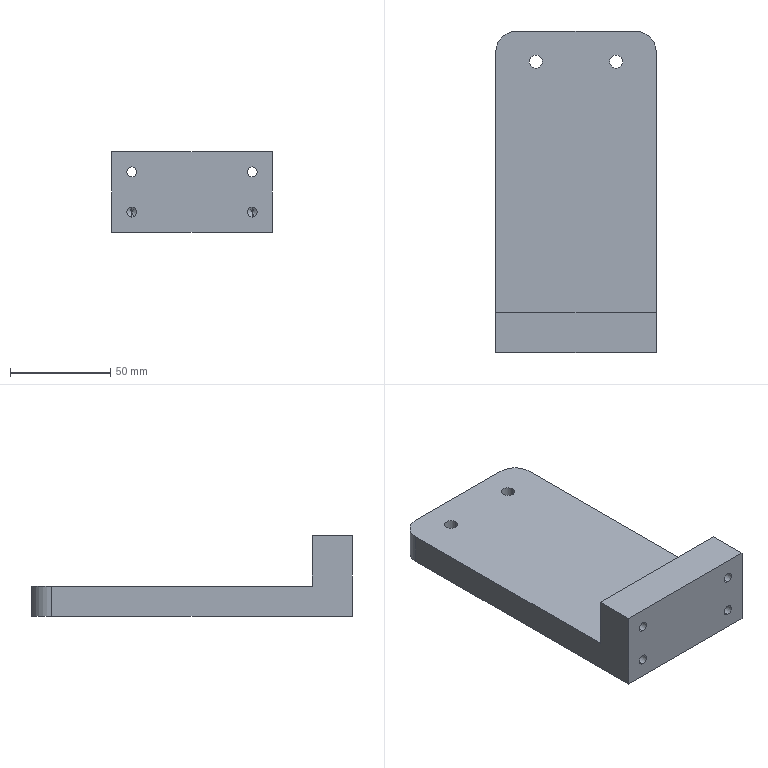Part | SolidWorks | features BaseBody 1 | 1 solid | 32 faces | box 80 x 160 x 40 mm | volume 227794 mm3 | cylinder 18 | plane 10 | cone 4 | commonest cylinder face diameters 5 x8 6.6 x4 11 x4 20 x2
STEP:
#1=CARTESIAN_POINT('',(25.5,65.,6.8));
#2=VERTEX_POINT('',#1);
#3=CARTESIAN_POINT('',(14.5,65.,6.8));
#4=VERTEX_POINT('',#3);
#5=CARTESIAN_POINT('',(20.,65.,6.8));
#6=DIRECTION('',(0.,0.,-1.));
#7=DIRECTION('',(-1.,0.,0.));
#8=AXIS2_PLACEMENT_3D('',#5,#6,#7);
#9=CIRCLE('',#8,5.5);
#10=EDGE_CURVE('',#2,#4,#9,.T.);
#11=ORIENTED_EDGE('',*,*,#10,.F.);
#12=CARTESIAN_POINT('',(25.5,65.,0.));
#13=VERTEX_POINT('',#12);
#14=CARTESIAN_POINT('',(25.5,65.,0.));
#15=DIRECTION('',(0.,0.,-1.));
#16=VECTOR('',#15,1000.);
#17=LINE('',#14,#16);
#18=EDGE_CURVE('',#2,#13,#17,.T.);
#19=ORIENTED_EDGE('',*,*,#18,.T.);
#20=CARTESIAN_POINT('',(14.5,65.,0.));
#21=VERTEX_POINT('',#20);
#22=CARTESIAN_POINT('',(20.,65.,0.));
#23=DIRECTION('',(0.,0.,-1.));
#24=DIRECTION('',(-1.,0.,0.));
#25=AXIS2_PLACEMENT_3D('',#22,#23,#24);
#26=CIRCLE('',#25,5.5);
#27=EDGE_CURVE('',#13,#21,#26,.T.);
#28=ORIENTED_EDGE('',*,*,#27,.T.);
#29=CARTESIAN_POINT('',(14.5,65.,0.));
#30=DIRECTION('',(0.,0.,-1.));
#31=VECTOR('',#30,1000.);
#32=LINE('',#29,#31);
#33=EDGE_CURVE('',#4,#21,#32,.T.);
#34=ORIENTED_EDGE('',*,*,#33,.F.);
#35=EDGE_LOOP('',(#11,#19,#28,#34));
#36=FACE_OUTER_BOUND('',#35,.T.);
#37=CARTESIAN_POINT('',(20.,65.,0.));
#38=DIRECTION('',(0.,0.,-1.));
#39=DIRECTION('',(-1.,0.,0.));
#40=AXIS2_PLACEMENT_3D('',#37,#38,#39);
#41=CYLINDRICAL_SURFACE('',#40,5.5);
#42=ADVANCED_FACE('',(#36),#41,.F.);
#43=CARTESIAN_POINT('',(23.3,65.,15.));
#44=VERTEX_POINT('',#43);
#45=CARTESIAN_POINT('',(16.7,65.,15.));
#46=VERTEX_POINT('',#45);
#47=CARTESIAN_POINT('',(20.,65.,15.));
#48=DIRECTION('',(0.,0.,-1.));
#49=DIRECTION('',(-1.,0.,0.));
#50=AXIS2_PLACEMENT_3D('',#47,#48,#49);
#51=CIRCLE('',#50,3.3);
#52=EDGE_CURVE('',#44,#46,#51,.T.);
#53=ORIENTED_EDGE('',*,*,#52,.F.);
#54=CARTESIAN_POINT('',(23.3,65.,6.8));
#55=VERTEX_POINT('',#54);
#56=CARTESIAN_POINT('',(23.3,65.,0.));
#57=DIRECTION('',(0.,0.,-1.));
#58=VECTOR('',#57,1000.);
#59=LINE('',#56,#58);
#60=EDGE_CURVE('',#44,#55,#59,.T.);
#61=ORIENTED_EDGE('',*,*,#60,.T.);
#62=CARTESIAN_POINT('',(16.7,65.,6.8));
#63=VERTEX_POINT('',#62);
#64=CARTESIAN_POINT('',(20.,65.,6.8));
#65=DIRECTION('',(0.,0.,-1.));
#66=DIRECTION('',(-1.,0.,0.));
#67=AXIS2_PLACEMENT_3D('',#64,#65,#66);
#68=CIRCLE('',#67,3.3);
#69=EDGE_CURVE('',#55,#63,#68,.T.);
#70=ORIENTED_EDGE('',*,*,#69,.T.);
#71=CARTESIAN_POINT('',(16.7,65.,0.));
#72=DIRECTION('',(0.,0.,-1.));
#73=VECTOR('',#72,1000.);
#74=LINE('',#71,#73);
#75=EDGE_CURVE('',#46,#63,#74,.T.);
#76=ORIENTED_EDGE('',*,*,#75,.F.);
#77=EDGE_LOOP('',(#53,#61,#70,#76));
#78=FACE_OUTER_BOUND('',#77,.T.);
#79=CARTESIAN_POINT('',(20.,65.,0.));
#80=DIRECTION('',(0.,0.,-1.));
#81=DIRECTION('',(-1.,0.,0.));
#82=AXIS2_PLACEMENT_3D('',#79,#80,#81);
#83=CYLINDRICAL_SURFACE('',#82,3.3);
#84=ADVANCED_FACE('',(#78),#83,.F.);
#85=CARTESIAN_POINT('',(-14.5,65.,6.8));
#86=VERTEX_POINT('',#85);
#87=CARTESIAN_POINT('',(-25.5,65.,6.8));
#88=VERTEX_POINT('',#87);
#89=CARTESIAN_POINT('',(-20.,65.,6.8));
#90=DIRECTION('',(0.,0.,-1.));
#91=DIRECTION('',(-1.,0.,0.));
#92=AXIS2_PLACEMENT_3D('',#89,#90,#91);
#93=CIRCLE('',#92,5.5);
#94=EDGE_CURVE('',#86,#88,#93,.T.);
#95=ORIENTED_EDGE('',*,*,#94,.F.);
#96=CARTESIAN_POINT('',(-14.5,65.,0.));
#97=VERTEX_POINT('',#96);
#98=CARTESIAN_POINT('',(-14.5,65.,0.));
#99=DIRECTION('',(0.,0.,-1.));
#100=VECTOR('',#99,1000.);
#101=LINE('',#98,#100);
#102=EDGE_CURVE('',#86,#97,#101,.T.);
#103=ORIENTED_EDGE('',*,*,#102,.T.);
#104=CARTESIAN_POINT('',(-25.5,65.,0.));
#105=VERTEX_POINT('',#104);
#106=CARTESIAN_POINT('',(-20.,65.,0.));
#107=DIRECTION('',(0.,0.,-1.));
#108=DIRECTION('',(-1.,0.,0.));
#109=AXIS2_PLACEMENT_3D('',#106,#107,#108);
#110=CIRCLE('',#109,5.5);
#111=EDGE_CURVE('',#97,#105,#110,.T.);
#112=ORIENTED_EDGE('',*,*,#111,.T.);
#113=CARTESIAN_POINT('',(-25.5,65.,0.));
#114=DIRECTION('',(0.,0.,-1.));
#115=VECTOR('',#114,1000.);
#116=LINE('',#113,#115);
#117=EDGE_CURVE('',#88,#105,#116,.T.);
#118=ORIENTED_EDGE('',*,*,#117,.F.);
#119=EDGE_LOOP('',(#95,#103,#112,#118));
#120=FACE_OUTER_BOUND('',#119,.T.);
#121=CARTESIAN_POINT('',(-20.,65.,0.));
#122=DIRECTION('',(0.,0.,-1.));
#123=DIRECTION('',(-1.,0.,0.));
#124=AXIS2_PLACEMENT_3D('',#121,#122,#123);
#125=CYLINDRICAL_SURFACE('',#124,5.5);
#126=ADVANCED_FACE('',(#120),#125,.F.);
#127=CARTESIAN_POINT('',(-16.7,65.,15.));
#128=VERTEX_POINT('',#127);
#129=CARTESIAN_POINT('',(-23.3,65.,15.));
#130=VERTEX_POINT('',#129);
#131=CARTESIAN_POINT('',(-20.,65.,15.));
#132=DIRECTION('',(0.,0.,-1.));
#133=DIRECTION('',(-1.,0.,0.));
#134=AXIS2_PLACEMENT_3D('',#131,#132,#133);
#135=CIRCLE('',#134,3.3);
#136=EDGE_CURVE('',#128,#130,#135,.T.);
#137=ORIENTED_EDGE('',*,*,#136,.F.);
#138=CARTESIAN_POINT('',(-16.7,65.,6.8));
#139=VERTEX_POINT('',#138);
#140=CARTESIAN_POINT('',(-16.7,65.,0.));
#141=DIRECTION('',(0.,0.,-1.));
#142=VECTOR('',#141,1000.);
#143=LINE('',#140,#142);
#144=EDGE_CURVE('',#128,#139,#143,.T.);
#145=ORIENTED_EDGE('',*,*,#144,.T.);
#146=CARTESIAN_POINT('',(-23.3,65.,6.8));
#147=VERTEX_POINT('',#146);
#148=CARTESIAN_POINT('',(-20.,65.,6.8));
#149=DIRECTION('',(0.,0.,-1.));
#150=DIRECTION('',(-1.,0.,0.));
#151=AXIS2_PLACEMENT_3D('',#148,#149,#150);
#152=CIRCLE('',#151,3.3);
#153=EDGE_CURVE('',#139,#147,#152,.T.);
#154=ORIENTED_EDGE('',*,*,#153,.T.);
#155=CARTESIAN_POINT('',(-23.3,65.,0.));
#156=DIRECTION('',(0.,0.,-1.));
#157=VECTOR('',#156,1000.);
#158=LINE('',#155,#157);
#159=EDGE_CURVE('',#130,#147,#158,.T.);
#160=ORIENTED_EDGE('',*,*,#159,.F.);
#161=EDGE_LOOP('',(#137,#145,#154,#160));
#162=FACE_OUTER_BOUND('',#161,.T.);
#163=CARTESIAN_POINT('',(-20.,65.,0.));
#164=DIRECTION('',(0.,0.,-1.));
#165=DIRECTION('',(-1.,0.,0.));
#166=AXIS2_PLACEMENT_3D('',#163,#164,#165);
#167=CYLINDRICAL_SURFACE('',#166,3.3);
#168=ADVANCED_FACE('',(#162),#167,.F.);
#169=CARTESIAN_POINT('',(30.,-60.,32.5));
#170=VERTEX_POINT('',#169);
#171=CARTESIAN_POINT('',(30.,-60.,27.5));
#172=VERTEX_POINT('',#171);
#173=CARTESIAN_POINT('',(30.,-60.,30.));
#174=DIRECTION('',(0.,-1.,0.));
#175=DIRECTION('',(0.,0.,-1.));
#176=AXIS2_PLACEMENT_3D('',#173,#174,#175);
#177=CIRCLE('',#176,2.5);
#178=EDGE_CURVE('',#170,#172,#177,.T.);
#179=ORIENTED_EDGE('',*,*,#178,.F.);
#180=CARTESIAN_POINT('',(30.,-80.,32.5));
#181=VERTEX_POINT('',#180);
#182=CARTESIAN_POINT('',(30.,-80.,32.5));
#183=DIRECTION('',(0.,-1.,0.));
#184=VECTOR('',#183,1000.);
#185=LINE('',#182,#184);
#186=EDGE_CURVE('',#170,#181,#185,.T.);
#187=ORIENTED_EDGE('',*,*,#186,.T.);
#188=CARTESIAN_POINT('',(30.,-80.,27.5));
#189=VERTEX_POINT('',#188);
#190=CARTESIAN_POINT('',(30.,-80.,30.));
#191=DIRECTION('',(0.,-1.,0.));
#192=DIRECTION('',(0.,0.,-1.));
#193=AXIS2_PLACEMENT_3D('',#190,#191,#192);
#194=CIRCLE('',#193,2.5);
#195=EDGE_CURVE('',#181,#189,#194,.T.);
#196=ORIENTED_EDGE('',*,*,#195,.T.);
#197=CARTESIAN_POINT('',(30.,-80.,27.5));
#198=DIRECTION('',(0.,-1.,0.));
#199=VECTOR('',#198,1000.);
#200=LINE('',#197,#199);
#201=EDGE_CURVE('',#172,#189,#200,.T.);
#202=ORIENTED_EDGE('',*,*,#201,.F.);
#203=EDGE_LOOP('',(#179,#187,#196,#202));
#204=FACE_OUTER_BOUND('',#203,.T.);
#205=CARTESIAN_POINT('',(30.,-80.,30.));
#206=DIRECTION('',(0.,-1.,0.));
#207=DIRECTION('',(0.,0.,-1.));
#208=AXIS2_PLACEMENT_3D('',#205,#206,#207);
#209=CYLINDRICAL_SURFACE('',#208,2.5);
#210=ADVANCED_FACE('',(#204),#209,.F.);
#211=CARTESIAN_POINT('',(30.,-57.,12.5));
#212=VERTEX_POINT('',#211);
#213=CARTESIAN_POINT('',(30.,-57.,7.5));
#214=VERTEX_POINT('',#213);
#215=CARTESIAN_POINT('',(30.,-57.,10.));
#216=DIRECTION('',(0.,-1.,0.));
#217=DIRECTION('',(0.,0.,-1.));
#218=AXIS2_PLACEMENT_3D('',#215,#216,#217);
#219=CIRCLE('',#218,2.5);
#220=EDGE_CURVE('',#212,#214,#219,.T.);
#221=ORIENTED_EDGE('',*,*,#220,.F.);
#222=CARTESIAN_POINT('',(30.,-80.,12.5));
#223=VERTEX_POINT('',#222);
#224=CARTESIAN_POINT('',(30.,-80.,12.5));
#225=DIRECTION('',(0.,-1.,0.));
#226=VECTOR('',#225,1000.);
#227=LINE('',#224,#226);
#228=EDGE_CURVE('',#212,#223,#227,.T.);
#229=ORIENTED_EDGE('',*,*,#228,.T.);
#230=CARTESIAN_POINT('',(30.,-80.,7.5));
#231=VERTEX_POINT('',#230);
#232=CARTESIAN_POINT('',(30.,-80.,10.));
#233=DIRECTION('',(0.,-1.,0.));
#234=DIRECTION('',(0.,0.,-1.));
#235=AXIS2_PLACEMENT_3D('',#232,#233,#234);
#236=CIRCLE('',#235,2.5);
#237=EDGE_CURVE('',#223,#231,#236,.T.);
#238=ORIENTED_EDGE('',*,*,#237,.T.);
#239=CARTESIAN_POINT('',(30.,-80.,7.5));
#240=DIRECTION('',(0.,-1.,0.));
#241=VECTOR('',#240,1000.);
#242=LINE('',#239,#241);
#243=EDGE_CURVE('',#214,#231,#242,.T.);
#244=ORIENTED_EDGE('',*,*,#243,.F.);
#245=EDGE_LOOP('',(#221,#229,#238,#244));
#246=FACE_OUTER_BOUND('',#245,.T.);
#247=CARTESIAN_POINT('',(30.,-80.,10.));
#248=DIRECTION('',(0.,-1.,0.));
#249=DIRECTION('',(0.,0.,-1.));
#250=AXIS2_PLACEMENT_3D('',#247,#248,#249);
#251=CYLINDRICAL_SURFACE('',#250,2.5);
#252=ADVANCED_FACE('',(#246),#251,.F.);
#253=CARTESIAN_POINT('',(30.,-55.498,10.));
#254=VERTEX_POINT('',#253);
#255=CARTESIAN_POINT('',(30.,-57.,7.5));
#256=DIRECTION('',(0.,-0.515,-0.8572));
#257=VECTOR('',#256,1000.);
#258=LINE('',#255,#257);
#259=EDGE_CURVE('',#254,#214,#258,.T.);
#260=ORIENTED_EDGE('',*,*,#259,.F.);
#261=CARTESIAN_POINT('',(30.,-57.,12.5));
#262=DIRECTION('',(0.,-0.515,0.8572));
#263=VECTOR('',#262,1000.);
#264=LINE('',#261,#263);
#265=EDGE_CURVE('',#254,#212,#264,.T.);
#266=ORIENTED_EDGE('',*,*,#265,.T.);
#267=ORIENTED_EDGE('',*,*,#220,.T.);
#268=EDGE_LOOP('',(#260,#266,#267));
#269=FACE_OUTER_BOUND('',#268,.T.);
#270=CARTESIAN_POINT('',(30.,-57.,10.));
#271=DIRECTION('',(0.,-1.,0.));
#272=DIRECTION('',(0.,0.,-1.));
#273=AXIS2_PLACEMENT_3D('',#270,#271,#272);
#274=CONICAL_SURFACE('',#273,2.5,1.03);
#275=ADVANCED_FACE('',(#269),#274,.F.);
#276=CARTESIAN_POINT('',(-30.,-57.,12.5));
#277=VERTEX_POINT('',#276);
#278=CARTESIAN_POINT('',(-30.,-57.,7.5));
#279=VERTEX_POINT('',#278);
#280=CARTESIAN_POINT('',(-30.,-57.,10.));
#281=DIRECTION('',(0.,-1.,0.));
#282=DIRECTION('',(0.,0.,-1.));
#283=AXIS2_PLACEMENT_3D('',#280,#281,#282);
#284=CIRCLE('',#283,2.5);
#285=EDGE_CURVE('',#277,#279,#284,.T.);
#286=ORIENTED_EDGE('',*,*,#285,.F.);
#287=CARTESIAN_POINT('',(-30.,-80.,12.5));
#288=VERTEX_POINT('',#287);
#289=CARTESIAN_POINT('',(-30.,-80.,12.5));
#290=DIRECTION('',(0.,-1.,0.));
#291=VECTOR('',#290,1000.);
#292=LINE('',#289,#291);
#293=EDGE_CURVE('',#277,#288,#292,.T.);
#294=ORIENTED_EDGE('',*,*,#293,.T.);
#295=CARTESIAN_POINT('',(-30.,-80.,7.5));
#296=VERTEX_POINT('',#295);
#297=CARTESIAN_POINT('',(-30.,-80.,10.));
#298=DIRECTION('',(0.,-1.,0.));
#299=DIRECTION('',(0.,0.,-1.));
#300=AXIS2_PLACEMENT_3D('',#297,#298,#299);
#301=CIRCLE('',#300,2.5);
#302=EDGE_CURVE('',#288,#296,#301,.T.);
#303=ORIENTED_EDGE('',*,*,#302,.T.);
#304=CARTESIAN_POINT('',(-30.,-80.,7.5));
#305=DIRECTION('',(0.,-1.,0.));
#306=VECTOR('',#305,1000.);
#307=LINE('',#304,#306);
#308=EDGE_CURVE('',#279,#296,#307,.T.);
#309=ORIENTED_EDGE('',*,*,#308,.F.);
#310=EDGE_LOOP('',(#286,#294,#303,#309));
#311=FACE_OUTER_BOUND('',#310,.T.);
#312=CARTESIAN_POINT('',(-30.,-80.,10.));
#313=DIRECTION('',(0.,-1.,0.));
#314=DIRECTION('',(0.,0.,-1.));
#315=AXIS2_PLACEMENT_3D('',#312,#313,#314);
#316=CYLINDRICAL_SURFACE('',#315,2.5);
#317=ADVANCED_FACE('',(#311),#316,.F.);
#318=CARTESIAN_POINT('',(-30.,-55.498,10.));
#319=VERTEX_POINT('',#318);
#320=CARTESIAN_POINT('',(-30.,-57.,7.5));
#321=DIRECTION('',(0.,-0.515,-0.8572));
#322=VECTOR('',#321,1000.);
#323=LINE('',#320,#322);
#324=EDGE_CURVE('',#319,#279,#323,.T.);
#325=ORIENTED_EDGE('',*,*,#324,.F.);
#326=CARTESIAN_POINT('',(-30.,-57.,12.5));
#327=DIRECTION('',(0.,-0.515,0.8572));
#328=VECTOR('',#327,1000.);
#329=LINE('',#326,#328);
#330=EDGE_CURVE('',#319,#277,#329,.T.);
#331=ORIENTED_EDGE('',*,*,#330,.T.);
#332=ORIENTED_EDGE('',*,*,#285,.T.);
#333=EDGE_LOOP('',(#325,#331,#332));
#334=FACE_OUTER_BOUND('',#333,.T.);
#335=CARTESIAN_POINT('',(-30.,-57.,10.));
#336=DIRECTION('',(0.,-1.,0.));
#337=DIRECTION('',(0.,0.,-1.));
#338=AXIS2_PLACEMENT_3D('',#335,#336,#337);
#339=CONICAL_SURFACE('',#338,2.5,1.03);
#340=ADVANCED_FACE('',(#334),#339,.F.);
#341=CARTESIAN_POINT('',(-30.,-60.,32.5));
#342=VERTEX_POINT('',#341);
#343=CARTESIAN_POINT('',(-30.,-60.,27.5));
#344=VERTEX_POINT('',#343);
#345=CARTESIAN_POINT('',(-30.,-60.,30.));
#346=DIRECTION('',(0.,-1.,0.));
#347=DIRECTION('',(0.,0.,-1.));
#348=AXIS2_PLACEMENT_3D('',#345,#346,#347);
#349=CIRCLE('',#348,2.5);
#350=EDGE_CURVE('',#342,#344,#349,.T.);
#351=ORIENTED_EDGE('',*,*,#350,.F.);
#352=CARTESIAN_POINT('',(-30.,-80.,32.5));
#353=VERTEX_POINT('',#352);
#354=CARTESIAN_POINT('',(-30.,-80.,32.5));
#355=DIRECTION('',(0.,-1.,0.));
#356=VECTOR('',#355,1000.);
#357=LINE('',#354,#356);
#358=EDGE_CURVE('',#342,#353,#357,.T.);
#359=ORIENTED_EDGE('',*,*,#358,.T.);
#360=CARTESIAN_POINT('',(-30.,-80.,27.5));
#361=VERTEX_POINT('',#360);
#362=CARTESIAN_POINT('',(-30.,-80.,30.));
#363=DIRECTION('',(0.,-1.,0.));
#364=DIRECTION('',(0.,0.,-1.));
#365=AXIS2_PLACEMENT_3D('',#362,#363,#364);
#366=CIRCLE('',#365,2.5);
#367=EDGE_CURVE('',#353,#361,#366,.T.);
#368=ORIENTED_EDGE('',*,*,#367,.T.);
#369=CARTESIAN_POINT('',(-30.,-80.,27.5));
#370=DIRECTION('',(0.,-1.,0.));
#371=VECTOR('',#370,1000.);
#372=LINE('',#369,#371);
#373=EDGE_CURVE('',#344,#361,#372,.T.);
#374=ORIENTED_EDGE('',*,*,#373,.F.);
#375=EDGE_LOOP('',(#351,#359,#368,#374));
#376=FACE_OUTER_BOUND('',#375,.T.);
#377=CARTESIAN_POINT('',(-30.,-80.,30.));
#378=DIRECTION('',(0.,-1.,0.));
#379=DIRECTION('',(0.,0.,-1.));
#380=AXIS2_PLACEMENT_3D('',#377,#378,#379);
#381=CYLINDRICAL_SURFACE('',#380,2.5);
#382=ADVANCED_FACE('',(#376),#381,.F.);
#383=CARTESIAN_POINT('',(20.,65.,6.8));
#384=DIRECTION('',(0.,0.,-1.));
#385=DIRECTION('',(-1.,0.,0.));
#386=AXIS2_PLACEMENT_3D('',#383,#384,#385);
#387=CIRCLE('',#386,3.3);
#388=EDGE_CURVE('',#63,#55,#387,.T.);
#389=ORIENTED_EDGE('',*,*,#388,.F.);
#390=ORIENTED_EDGE('',*,*,#69,.F.);
#391=EDGE_LOOP('',(#389,#390));
#392=FACE_BOUND('',#391,.T.);
#393=CARTESIAN_POINT('',(20.,65.,6.8));
#394=DIRECTION('',(0.,0.,-1.));
#395=DIRECTION('',(-1.,0.,0.));
#396=AXIS2_PLACEMENT_3D('',#393,#394,#395);
#397=CIRCLE('',#396,5.5);
#398=EDGE_CURVE('',#4,#2,#397,.T.);
#399=ORIENTED_EDGE('',*,*,#398,.T.);
#400=ORIENTED_EDGE('',*,*,#10,.T.);
#401=EDGE_LOOP('',(#399,#400));
#402=FACE_OUTER_BOUND('',#401,.T.);
#403=CARTESIAN_POINT('',(23.3,65.,6.8));
#404=DIRECTION('',(0.,0.,1.));
#405=DIRECTION('',(1.,0.,0.));
#406=AXIS2_PLACEMENT_3D('',#403,#404,#405);
#407=PLANE('',#406);
#408=ADVANCED_FACE('',(#392,#402),#407,.F.);
#409=CARTESIAN_POINT('',(-20.,65.,6.8));
#410=DIRECTION('',(0.,0.,-1.));
#411=DIRECTION('',(-1.,0.,0.));
#412=AXIS2_PLACEMENT_3D('',#409,#410,#411);
#413=CIRCLE('',#412,3.3);
#414=EDGE_CURVE('',#147,#139,#413,.T.);
#415=ORIENTED_EDGE('',*,*,#414,.F.);
#416=ORIENTED_EDGE('',*,*,#153,.F.);
#417=EDGE_LOOP('',(#415,#416));
#418=FACE_BOUND('',#417,.T.);
#419=CARTESIAN_POINT('',(-20.,65.,6.8));
#420=DIRECTION('',(0.,0.,-1.));
#421=DIRECTION('',(-1.,0.,0.));
#422=AXIS2_PLACEMENT_3D('',#419,#420,#421);
#423=CIRCLE('',#422,5.5);
#424=EDGE_CURVE('',#88,#86,#423,.T.);
#425=ORIENTED_EDGE('',*,*,#424,.T.);
#426=ORIENTED_EDGE('',*,*,#94,.T.);
#427=EDGE_LOOP('',(#425,#426));
#428=FACE_OUTER_BOUND('',#427,.T.);
#429=CARTESIAN_POINT('',(-16.7,65.,6.8));
#430=DIRECTION('',(0.,0.,1.));
#431=DIRECTION('',(1.,0.,0.));
#432=AXIS2_PLACEMENT_3D('',#429,#430,#431);
#433=PLANE('',#432);
#434=ADVANCED_FACE('',(#418,#428),#433,.F.);
#435=CARTESIAN_POINT('',(40.,70.,15.));
#436=VERTEX_POINT('',#435);
#437=CARTESIAN_POINT('',(30.,80.,15.));
#438=VERTEX_POINT('',#437);
#439=CARTESIAN_POINT('',(30.,70.,15.));
#440=DIRECTION('',(0.,0.,1.));
#441=DIRECTION('',(-1.,0.,0.));
#442=AXIS2_PLACEMENT_3D('',#439,#440,#441);
#443=CIRCLE('',#442,10.);
#444=EDGE_CURVE('',#436,#438,#443,.T.);
#445=ORIENTED_EDGE('',*,*,#444,.F.);
#446=CARTESIAN_POINT('',(40.,70.,0.));
#447=VERTEX_POINT('',#446);
#448=CARTESIAN_POINT('',(40.,70.,40.));
#449=DIRECTION('',(0.,0.,1.));
#450=VECTOR('',#449,1000.);
#451=LINE('',#448,#450);
#452=EDGE_CURVE('',#447,#436,#451,.T.);
#453=ORIENTED_EDGE('',*,*,#452,.F.);
#454=CARTESIAN_POINT('',(30.,80.,0.));
#455=VERTEX_POINT('',#454);
#456=CARTESIAN_POINT('',(30.,70.,0.));
#457=DIRECTION('',(0.,0.,-1.));
#458=DIRECTION('',(1.,0.,0.));
#459=AXIS2_PLACEMENT_3D('',#456,#457,#458);
#460=CIRCLE('',#459,10.);
#461=EDGE_CURVE('',#455,#447,#460,.T.);
#462=ORIENTED_EDGE('',*,*,#461,.F.);
#463=CARTESIAN_POINT('',(30.,80.,40.));
#464=DIRECTION('',(0.,0.,-1.));
#465=VECTOR('',#464,1000.);
#466=LINE('',#463,#465);
#467=EDGE_CURVE('',#438,#455,#466,.T.);
#468=ORIENTED_EDGE('',*,*,#467,.F.);
#469=EDGE_LOOP('',(#445,#453,#462,#468));
#470=FACE_OUTER_BOUND('',#469,.T.);
#471=CARTESIAN_POINT('',(30.,70.,40.));
#472=DIRECTION('',(0.,0.,-1.));
#473=DIRECTION('',(-1.,0.,0.));
#474=AXIS2_PLACEMENT_3D('',#471,#472,#473);
#475=CYLINDRICAL_SURFACE('',#474,10.);
#476=ADVANCED_FACE('',(#470),#475,.T.);
#477=CARTESIAN_POINT('',(-30.,80.,15.));
#478=VERTEX_POINT('',#477);
#479=CARTESIAN_POINT('',(-40.,70.,15.));
#480=VERTEX_POINT('',#479);
#481=CARTESIAN_POINT('',(-30.,70.,15.));
#482=DIRECTION('',(0.,0.,1.));
#483=DIRECTION('',(-1.,0.,0.));
#484=AXIS2_PLACEMENT_3D('',#481,#482,#483);
#485=CIRCLE('',#484,10.);
#486=EDGE_CURVE('',#478,#480,#485,.T.);
#487=ORIENTED_EDGE('',*,*,#486,.F.);
#488=CARTESIAN_POINT('',(-30.,80.,0.));
#489=VERTEX_POINT('',#488);
#490=CARTESIAN_POINT('',(-30.,80.,40.));
#491=DIRECTION('',(0.,0.,1.));
#492=VECTOR('',#491,1000.);
#493=LINE('',#490,#492);
#494=EDGE_CURVE('',#489,#478,#493,.T.);
#495=ORIENTED_EDGE('',*,*,#494,.F.);
#496=CARTESIAN_POINT('',(-40.,70.,0.));
#497=VERTEX_POINT('',#496);
#498=CARTESIAN_POINT('',(-30.,70.,0.));
#499=DIRECTION('',(0.,0.,-1.));
#500=DIRECTION('',(1.,0.,0.));
#501=AXIS2_PLACEMENT_3D('',#498,#499,#500);
#502=CIRCLE('',#501,10.);
#503=EDGE_CURVE('',#497,#489,#502,.T.);
#504=ORIENTED_EDGE('',*,*,#503,.F.);
#505=CARTESIAN_POINT('',(-40.,70.,40.));
#506=DIRECTION('',(0.,0.,-1.));
#507=VECTOR('',#506,1000.);
#508=LINE('',#505,#507);
#509=EDGE_CURVE('',#480,#497,#508,.T.);
#510=ORIENTED_EDGE('',*,*,#509,.F.);
#511=EDGE_LOOP('',(#487,#495,#504,#510));
#512=FACE_OUTER_BOUND('',#511,.T.);
#513=CARTESIAN_POINT('',(-30.,70.,40.));
#514=DIRECTION('',(0.,0.,-1.));
#515=DIRECTION('',(-1.,0.,0.));
#516=AXIS2_PLACEMENT_3D('',#513,#514,#515);
#517=CYLINDRICAL_SURFACE('',#516,10.);
#518=ADVANCED_FACE('',(#512),#517,.T.);
#519=CARTESIAN_POINT('',(-30.,-60.,30.));
#520=DIRECTION('',(0.,-1.,0.));
#521=DIRECTION('',(0.,0.,-1.));
#522=AXIS2_PLACEMENT_3D('',#519,#520,#521);
#523=CIRCLE('',#522,2.5);
#524=EDGE_CURVE('',#344,#342,#523,.T.);
#525=ORIENTED_EDGE('',*,*,#524,.T.);
#526=ORIENTED_EDGE('',*,*,#350,.T.);
#527=EDGE_LOOP('',(#525,#526));
#528=FACE_BOUND('',#527,.T.);
#529=CARTESIAN_POINT('',(30.,-60.,30.));
#530=DIRECTION('',(0.,-1.,0.));
#531=DIRECTION('',(0.,0.,-1.));
#532=AXIS2_PLACEMENT_3D('',#529,#530,#531);
#533=CIRCLE('',#532,2.5);
#534=EDGE_CURVE('',#172,#170,#533,.T.);
#535=ORIENTED_EDGE('',*,*,#534,.T.);
#536=ORIENTED_EDGE('',*,*,#178,.T.);
#537=EDGE_LOOP('',(#535,#536));
#538=FACE_BOUND('',#537,.T.);
#539=CARTESIAN_POINT('',(-40.,-60.,15.));
#540=VERTEX_POINT('',#539);
#541=CARTESIAN_POINT('',(-40.,-60.,40.));
#542=VERTEX_POINT('',#541);
#543=CARTESIAN_POINT('',(-40.,-60.,40.));
#544=DIRECTION('',(0.,0.,1.));
#545=VECTOR('',#544,1000.);
#546=LINE('',#543,#545);
#547=EDGE_CURVE('',#540,#542,#546,.T.);
#548=ORIENTED_EDGE('',*,*,#547,.T.);
#549=CARTESIAN_POINT('',(40.,-60.,40.));
#550=VERTEX_POINT('',#549);
#551=CARTESIAN_POINT('',(-40.,-60.,40.));
#552=DIRECTION('',(1.,0.,0.));
#553=VECTOR('',#552,1000.);
#554=LINE('',#551,#553);
#555=EDGE_CURVE('',#542,#550,#554,.T.);
#556=ORIENTED_EDGE('',*,*,#555,.T.);
#557=CARTESIAN_POINT('',(40.,-60.,15.));
#558=VERTEX_POINT('',#557);
#559=CARTESIAN_POINT('',(40.,-60.,40.));
#560=DIRECTION('',(0.,0.,-1.));
#561=VECTOR('',#560,1000.);
#562=LINE('',#559,#561);
#563=EDGE_CURVE('',#550,#558,#562,.T.);
#564=ORIENTED_EDGE('',*,*,#563,.T.);
#565=CARTESIAN_POINT('',(-40.,-60.,15.));
#566=DIRECTION('',(-1.,0.,0.));
#567=VECTOR('',#566,1000.);
#568=LINE('',#565,#567);
#569=EDGE_CURVE('',#558,#540,#568,.T.);
#570=ORIENTED_EDGE('',*,*,#569,.T.);
#571=EDGE_LOOP('',(#548,#556,#564,#570));
#572=FACE_OUTER_BOUND('',#571,.T.);
#573=CARTESIAN_POINT('',(0.,-60.,0.));
#574=DIRECTION('',(0.,-1.,0.));
#575=DIRECTION('',(0.,0.,-1.));
#576=AXIS2_PLACEMENT_3D('',#573,#574,#575);
#577=PLANE('',#576);
#578=ADVANCED_FACE('',(#528,#538,#572),#577,.F.);
#579=CARTESIAN_POINT('',(-20.,65.,15.));
#580=DIRECTION('',(0.,0.,-1.));
#581=DIRECTION('',(-1.,0.,0.));
#582=AXIS2_PLACEMENT_3D('',#579,#580,#581);
#583=CIRCLE('',#582,3.3);
#584=EDGE_CURVE('',#130,#128,#583,.T.);
#585=ORIENTED_EDGE('',*,*,#584,.T.);
#586=ORIENTED_EDGE('',*,*,#136,.T.);
#587=EDGE_LOOP('',(#585,#586));
#588=FACE_BOUND('',#587,.T.);
#589=CARTESIAN_POINT('',(20.,65.,15.));
#590=DIRECTION('',(0.,0.,-1.));
#591=DIRECTION('',(-1.,0.,0.));
#592=AXIS2_PLACEMENT_3D('',#589,#590,#591);
#593=CIRCLE('',#592,3.3);
#594=EDGE_CURVE('',#46,#44,#593,.T.);
#595=ORIENTED_EDGE('',*,*,#594,.T.);
#596=ORIENTED_EDGE('',*,*,#52,.T.);
#597=EDGE_LOOP('',(#595,#596));
#598=FACE_BOUND('',#597,.T.);
#599=CARTESIAN_POINT('',(-40.,80.,15.));
#600=DIRECTION('',(-1.,0.,0.));
#601=VECTOR('',#600,1000.);
#602=LINE('',#599,#601);
#603=EDGE_CURVE('',#438,#478,#602,.T.);
#604=ORIENTED_EDGE('',*,*,#603,.T.);
#605=ORIENTED_EDGE('',*,*,#486,.T.);
#606=CARTESIAN_POINT('',(-40.,-60.,15.));
#607=DIRECTION('',(0.,1.,0.));
#608=VECTOR('',#607,1000.);
#609=LINE('',#606,#608);
#610=EDGE_CURVE('',#540,#480,#609,.T.);
#611=ORIENTED_EDGE('',*,*,#610,.F.);
#612=ORIENTED_EDGE('',*,*,#569,.F.);
#613=CARTESIAN_POINT('',(40.,-60.,15.));
#614=DIRECTION('',(0.,1.,0.));
#615=VECTOR('',#614,1000.);
#616=LINE('',#613,#615);
#617=EDGE_CURVE('',#558,#436,#616,.T.);
#618=ORIENTED_EDGE('',*,*,#617,.T.);
#619=ORIENTED_EDGE('',*,*,#444,.T.);
#620=EDGE_LOOP('',(#604,#605,#611,#612,#618,#619));
#621=FACE_OUTER_BOUND('',#620,.T.);
#622=CARTESIAN_POINT('',(-40.,-60.,15.));
#623=DIRECTION('',(0.,0.,-1.));
#624=DIRECTION('',(0.,-1.,0.));
#625=AXIS2_PLACEMENT_3D('',#622,#623,#624);
#626=PLANE('',#625);
#627=ADVANCED_FACE('',(#588,#598,#621),#626,.F.);
#628=CARTESIAN_POINT('',(-20.,65.,0.));
#629=DIRECTION('',(0.,0.,-1.));
#630=DIRECTION('',(-1.,0.,0.));
#631=AXIS2_PLACEMENT_3D('',#628,#629,#630);
#632=CIRCLE('',#631,5.5);
#633=EDGE_CURVE('',#105,#97,#632,.T.);
#634=ORIENTED_EDGE('',*,*,#633,.F.);
#635=ORIENTED_EDGE('',*,*,#111,.F.);
#636=EDGE_LOOP('',(#634,#635));
#637=FACE_BOUND('',#636,.T.);
#638=CARTESIAN_POINT('',(20.,65.,0.));
#639=DIRECTION('',(0.,0.,-1.));
#640=DIRECTION('',(-1.,0.,0.));
#641=AXIS2_PLACEMENT_3D('',#638,#639,#640);
#642=CIRCLE('',#641,5.5);
#643=EDGE_CURVE('',#21,#13,#642,.T.);
#644=ORIENTED_EDGE('',*,*,#643,.F.);
#645=ORIENTED_EDGE('',*,*,#27,.F.);
#646=EDGE_LOOP('',(#644,#645));
#647=FACE_BOUND('',#646,.T.);
#648=CARTESIAN_POINT('',(-40.,-80.,0.));
#649=VERTEX_POINT('',#648);
#650=CARTESIAN_POINT('',(-40.,80.,0.));
#651=DIRECTION('',(0.,-1.,0.));
#652=VECTOR('',#651,1000.);
#653=LINE('',#650,#652);
#654=EDGE_CURVE('',#497,#649,#653,.T.);
#655=ORIENTED_EDGE('',*,*,#654,.F.);
#656=ORIENTED_EDGE('',*,*,#503,.T.);
#657=CARTESIAN_POINT('',(-40.,80.,0.));
#658=DIRECTION('',(-1.,0.,0.));
#659=VECTOR('',#658,1000.);
#660=LINE('',#657,#659);
#661=EDGE_CURVE('',#455,#489,#660,.T.);
#662=ORIENTED_EDGE('',*,*,#661,.F.);
#663=ORIENTED_EDGE('',*,*,#461,.T.);
#664=CARTESIAN_POINT('',(40.,-80.,0.));
#665=VERTEX_POINT('',#664);
#666=CARTESIAN_POINT('',(40.,80.,0.));
#667=DIRECTION('',(0.,1.,0.));
#668=VECTOR('',#667,1000.);
#669=LINE('',#666,#668);
#670=EDGE_CURVE('',#665,#447,#669,.T.);
#671=ORIENTED_EDGE('',*,*,#670,.F.);
#672=CARTESIAN_POINT('',(-40.,-80.,0.));
#673=DIRECTION('',(1.,0.,0.));
#674=VECTOR('',#673,1000.);
#675=LINE('',#672,#674);
#676=EDGE_CURVE('',#649,#665,#675,.T.);
#677=ORIENTED_EDGE('',*,*,#676,.F.);
#678=EDGE_LOOP('',(#655,#656,#662,#663,#671,#677));
#679=FACE_OUTER_BOUND('',#678,.T.);
#680=CARTESIAN_POINT('',(0.,0.,0.));
#681=DIRECTION('',(0.,0.,1.));
#682=DIRECTION('',(1.,0.,0.));
#683=AXIS2_PLACEMENT_3D('',#680,#681,#682);
#684=PLANE('',#683);
#685=ADVANCED_FACE('',(#637,#647,#679),#684,.F.);
#686=ORIENTED_EDGE('',*,*,#555,.F.);
#687=CARTESIAN_POINT('',(-40.,-80.,40.));
#688=VERTEX_POINT('',#687);
#689=CARTESIAN_POINT('',(-40.,80.,40.));
#690=DIRECTION('',(0.,-1.,0.));
#691=VECTOR('',#690,1000.);
#692=LINE('',#689,#691);
#693=EDGE_CURVE('',#542,#688,#692,.T.);
#694=ORIENTED_EDGE('',*,*,#693,.T.);
#695=CARTESIAN_POINT('',(40.,-80.,40.));
#696=VERTEX_POINT('',#695);
#697=CARTESIAN_POINT('',(-40.,-80.,40.));
#698=DIRECTION('',(1.,0.,0.));
#699=VECTOR('',#698,1000.);
#700=LINE('',#697,#699);
#701=EDGE_CURVE('',#688,#696,#700,.T.);
#702=ORIENTED_EDGE('',*,*,#701,.T.);
#703=CARTESIAN_POINT('',(40.,80.,40.));
#704=DIRECTION('',(0.,1.,0.));
#705=VECTOR('',#704,1000.);
#706=LINE('',#703,#705);
#707=EDGE_CURVE('',#696,#550,#706,.T.);
#708=ORIENTED_EDGE('',*,*,#707,.T.);
#709=EDGE_LOOP('',(#686,#694,#702,#708));
#710=FACE_OUTER_BOUND('',#709,.T.);
#711=CARTESIAN_POINT('',(0.,0.,40.));
#712=DIRECTION('',(0.,0.,1.));
#713=DIRECTION('',(1.,0.,0.));
#714=AXIS2_PLACEMENT_3D('',#711,#712,#713);
#715=PLANE('',#714);
#716=ADVANCED_FACE('',(#710),#715,.T.);
#717=CARTESIAN_POINT('',(-30.,-80.,30.));
#718=DIRECTION('',(0.,-1.,0.));
#719=DIRECTION('',(0.,0.,-1.));
#720=AXIS2_PLACEMENT_3D('',#717,#718,#719);
#721=CIRCLE('',#720,2.5);
#722=EDGE_CURVE('',#361,#353,#721,.T.);
#723=ORIENTED_EDGE('',*,*,#722,.F.);
#724=ORIENTED_EDGE('',*,*,#367,.F.);
#725=EDGE_LOOP('',(#723,#724));
#726=FACE_BOUND('',#725,.T.);
#727=CARTESIAN_POINT('',(-30.,-80.,10.));
#728=DIRECTION('',(0.,-1.,0.));
#729=DIRECTION('',(0.,0.,-1.));
#730=AXIS2_PLACEMENT_3D('',#727,#728,#729);
#731=CIRCLE('',#730,2.5);
#732=EDGE_CURVE('',#296,#288,#731,.T.);
#733=ORIENTED_EDGE('',*,*,#732,.F.);
#734=ORIENTED_EDGE('',*,*,#302,.F.);
#735=EDGE_LOOP('',(#733,#734));
#736=FACE_BOUND('',#735,.T.);
#737=CARTESIAN_POINT('',(30.,-80.,10.));
#738=DIRECTION('',(0.,-1.,0.));
#739=DIRECTION('',(0.,0.,-1.));
#740=AXIS2_PLACEMENT_3D('',#737,#738,#739);
#741=CIRCLE('',#740,2.5);
#742=EDGE_CURVE('',#231,#223,#741,.T.);
#743=ORIENTED_EDGE('',*,*,#742,.F.);
#744=ORIENTED_EDGE('',*,*,#237,.F.);
#745=EDGE_LOOP('',(#743,#744));
#746=FACE_BOUND('',#745,.T.);
#747=CARTESIAN_POINT('',(30.,-80.,30.));
#748=DIRECTION('',(0.,-1.,0.));
#749=DIRECTION('',(0.,0.,-1.));
#750=AXIS2_PLACEMENT_3D('',#747,#748,#749);
#751=CIRCLE('',#750,2.5);
#752=EDGE_CURVE('',#189,#181,#751,.T.);
#753=ORIENTED_EDGE('',*,*,#752,.F.);
#754=ORIENTED_EDGE('',*,*,#195,.F.);
#755=EDGE_LOOP('',(#753,#754));
#756=FACE_BOUND('',#755,.T.);
#757=ORIENTED_EDGE('',*,*,#676,.T.);
#758=CARTESIAN_POINT('',(40.,-80.,40.));
#759=DIRECTION('',(0.,0.,-1.));
#760=VECTOR('',#759,1000.);
#761=LINE('',#758,#760);
#762=EDGE_CURVE('',#696,#665,#761,.T.);
#763=ORIENTED_EDGE('',*,*,#762,.F.);
#764=ORIENTED_EDGE('',*,*,#701,.F.);
#765=CARTESIAN_POINT('',(-40.,-80.,40.));
#766=DIRECTION('',(0.,0.,-1.));
#767=VECTOR('',#766,1000.);
#768=LINE('',#765,#767);
#769=EDGE_CURVE('',#688,#649,#768,.T.);
#770=ORIENTED_EDGE('',*,*,#769,.T.);
#771=EDGE_LOOP('',(#757,#763,#764,#770));
#772=FACE_OUTER_BOUND('',#771,.T.);
#773=CARTESIAN_POINT('',(-40.,-80.,40.));
#774=DIRECTION('',(0.,1.,0.));
#775=DIRECTION('',(1.,0.,0.));
#776=AXIS2_PLACEMENT_3D('',#773,#774,#775);
#777=PLANE('',#776);
#778=ADVANCED_FACE('',(#726,#736,#746,#756,#772),#777,.F.);
#779=ORIENTED_EDGE('',*,*,#610,.T.);
#780=ORIENTED_EDGE('',*,*,#509,.T.);
#781=ORIENTED_EDGE('',*,*,#654,.T.);
#782=ORIENTED_EDGE('',*,*,#769,.F.);
#783=ORIENTED_EDGE('',*,*,#693,.F.);
#784=ORIENTED_EDGE('',*,*,#547,.F.);
#785=EDGE_LOOP('',(#779,#780,#781,#782,#783,#784));
#786=FACE_OUTER_BOUND('',#785,.T.);
#787=CARTESIAN_POINT('',(-40.,80.,40.));
#788=DIRECTION('',(1.,0.,0.));
#789=DIRECTION('',(0.,1.,0.));
#790=AXIS2_PLACEMENT_3D('',#787,#788,#789);
#791=PLANE('',#790);
#792=ADVANCED_FACE('',(#786),#791,.F.);
#793=ORIENTED_EDGE('',*,*,#661,.T.);
#794=ORIENTED_EDGE('',*,*,#494,.T.);
#795=ORIENTED_EDGE('',*,*,#603,.F.);
#796=ORIENTED_EDGE('',*,*,#467,.T.);
#797=EDGE_LOOP('',(#793,#794,#795,#796));
#798=FACE_OUTER_BOUND('',#797,.T.);
#799=CARTESIAN_POINT('',(-40.,80.,40.));
#800=DIRECTION('',(0.,-1.,0.));
#801=DIRECTION('',(0.,0.,-1.));
#802=AXIS2_PLACEMENT_3D('',#799,#800,#801);
#803=PLANE('',#802);
#804=ADVANCED_FACE('',(#798),#803,.F.);
#805=ORIENTED_EDGE('',*,*,#670,.T.);
#806=ORIENTED_EDGE('',*,*,#452,.T.);
#807=ORIENTED_EDGE('',*,*,#617,.F.);
#808=ORIENTED_EDGE('',*,*,#563,.F.);
#809=ORIENTED_EDGE('',*,*,#707,.F.);
#810=ORIENTED_EDGE('',*,*,#762,.T.);
#811=EDGE_LOOP('',(#805,#806,#807,#808,#809,#810));
#812=FACE_OUTER_BOUND('',#811,.T.);
#813=CARTESIAN_POINT('',(40.,80.,40.));
#814=DIRECTION('',(-1.,0.,0.));
#815=DIRECTION('',(0.,1.,0.));
#816=AXIS2_PLACEMENT_3D('',#813,#814,#815);
#817=PLANE('',#816);
#818=ADVANCED_FACE('',(#812),#817,.F.);
#819=ORIENTED_EDGE('',*,*,#358,.F.);
#820=ORIENTED_EDGE('',*,*,#524,.F.);
#821=ORIENTED_EDGE('',*,*,#373,.T.);
#822=ORIENTED_EDGE('',*,*,#722,.T.);
#823=EDGE_LOOP('',(#819,#820,#821,#822));
#824=FACE_OUTER_BOUND('',#823,.T.);
#825=CARTESIAN_POINT('',(-30.,-80.,30.));
#826=DIRECTION('',(0.,-1.,0.));
#827=DIRECTION('',(0.,0.,-1.));
#828=AXIS2_PLACEMENT_3D('',#825,#826,#827);
#829=CYLINDRICAL_SURFACE('',#828,2.5);
#830=ADVANCED_FACE('',(#824),#829,.F.);
#831=ORIENTED_EDGE('',*,*,#330,.F.);
#832=ORIENTED_EDGE('',*,*,#324,.T.);
#833=CARTESIAN_POINT('',(-30.,-57.,10.));
#834=DIRECTION('',(0.,-1.,0.));
#835=DIRECTION('',(0.,0.,-1.));
#836=AXIS2_PLACEMENT_3D('',#833,#834,#835);
#837=CIRCLE('',#836,2.5);
#838=EDGE_CURVE('',#279,#277,#837,.T.);
#839=ORIENTED_EDGE('',*,*,#838,.T.);
#840=EDGE_LOOP('',(#831,#832,#839));
#841=FACE_OUTER_BOUND('',#840,.T.);
#842=CARTESIAN_POINT('',(-30.,-57.,10.));
#843=DIRECTION('',(0.,-1.,0.));
#844=DIRECTION('',(0.,0.,-1.));
#845=AXIS2_PLACEMENT_3D('',#842,#843,#844);
#846=CONICAL_SURFACE('',#845,2.5,1.03);
#847=ADVANCED_FACE('',(#841),#846,.F.);
#848=ORIENTED_EDGE('',*,*,#293,.F.);
#849=ORIENTED_EDGE('',*,*,#838,.F.);
#850=ORIENTED_EDGE('',*,*,#308,.T.);
#851=ORIENTED_EDGE('',*,*,#732,.T.);
#852=EDGE_LOOP('',(#848,#849,#850,#851));
#853=FACE_OUTER_BOUND('',#852,.T.);
#854=CARTESIAN_POINT('',(-30.,-80.,10.));
#855=DIRECTION('',(0.,-1.,0.));
#856=DIRECTION('',(0.,0.,-1.));
#857=AXIS2_PLACEMENT_3D('',#854,#855,#856);
#858=CYLINDRICAL_SURFACE('',#857,2.5);
#859=ADVANCED_FACE('',(#853),#858,.F.);
#860=ORIENTED_EDGE('',*,*,#265,.F.);
#861=ORIENTED_EDGE('',*,*,#259,.T.);
#862=CARTESIAN_POINT('',(30.,-57.,10.));
#863=DIRECTION('',(0.,-1.,0.));
#864=DIRECTION('',(0.,0.,-1.));
#865=AXIS2_PLACEMENT_3D('',#862,#863,#864);
#866=CIRCLE('',#865,2.5);
#867=EDGE_CURVE('',#214,#212,#866,.T.);
#868=ORIENTED_EDGE('',*,*,#867,.T.);
#869=EDGE_LOOP('',(#860,#861,#868));
#870=FACE_OUTER_BOUND('',#869,.T.);
#871=CARTESIAN_POINT('',(30.,-57.,10.));
#872=DIRECTION('',(0.,-1.,0.));
#873=DIRECTION('',(0.,0.,-1.));
#874=AXIS2_PLACEMENT_3D('',#871,#872,#873);
#875=CONICAL_SURFACE('',#874,2.5,1.03);
#876=ADVANCED_FACE('',(#870),#875,.F.);
#877=ORIENTED_EDGE('',*,*,#228,.F.);
#878=ORIENTED_EDGE('',*,*,#867,.F.);
#879=ORIENTED_EDGE('',*,*,#243,.T.);
#880=ORIENTED_EDGE('',*,*,#742,.T.);
#881=EDGE_LOOP('',(#877,#878,#879,#880));
#882=FACE_OUTER_BOUND('',#881,.T.);
#883=CARTESIAN_POINT('',(30.,-80.,10.));
#884=DIRECTION('',(0.,-1.,0.));
#885=DIRECTION('',(0.,0.,-1.));
#886=AXIS2_PLACEMENT_3D('',#883,#884,#885);
#887=CYLINDRICAL_SURFACE('',#886,2.5);
#888=ADVANCED_FACE('',(#882),#887,.F.);
#889=ORIENTED_EDGE('',*,*,#186,.F.);
#890=ORIENTED_EDGE('',*,*,#534,.F.);
#891=ORIENTED_EDGE('',*,*,#201,.T.);
#892=ORIENTED_EDGE('',*,*,#752,.T.);
#893=EDGE_LOOP('',(#889,#890,#891,#892));
#894=FACE_OUTER_BOUND('',#893,.T.);
#895=CARTESIAN_POINT('',(30.,-80.,30.));
#896=DIRECTION('',(0.,-1.,0.));
#897=DIRECTION('',(0.,0.,-1.));
#898=AXIS2_PLACEMENT_3D('',#895,#896,#897);
#899=CYLINDRICAL_SURFACE('',#898,2.5);
#900=ADVANCED_FACE('',(#894),#899,.F.);
#901=ORIENTED_EDGE('',*,*,#144,.F.);
#902=ORIENTED_EDGE('',*,*,#584,.F.);
#903=ORIENTED_EDGE('',*,*,#159,.T.);
#904=ORIENTED_EDGE('',*,*,#414,.T.);
#905=EDGE_LOOP('',(#901,#902,#903,#904));
#906=FACE_OUTER_BOUND('',#905,.T.);
#907=CARTESIAN_POINT('',(-20.,65.,0.));
#908=DIRECTION('',(0.,0.,-1.));
#909=DIRECTION('',(-1.,0.,0.));
#910=AXIS2_PLACEMENT_3D('',#907,#908,#909);
#911=CYLINDRICAL_SURFACE('',#910,3.3);
#912=ADVANCED_FACE('',(#906),#911,.F.);
#913=ORIENTED_EDGE('',*,*,#102,.F.);
#914=ORIENTED_EDGE('',*,*,#424,.F.);
#915=ORIENTED_EDGE('',*,*,#117,.T.);
#916=ORIENTED_EDGE('',*,*,#633,.T.);
#917=EDGE_LOOP('',(#913,#914,#915,#916));
#918=FACE_OUTER_BOUND('',#917,.T.);
#919=CARTESIAN_POINT('',(-20.,65.,0.));
#920=DIRECTION('',(0.,0.,-1.));
#921=DIRECTION('',(-1.,0.,0.));
#922=AXIS2_PLACEMENT_3D('',#919,#920,#921);
#923=CYLINDRICAL_SURFACE('',#922,5.5);
#924=ADVANCED_FACE('',(#918),#923,.F.);
#925=ORIENTED_EDGE('',*,*,#60,.F.);
#926=ORIENTED_EDGE('',*,*,#594,.F.);
#927=ORIENTED_EDGE('',*,*,#75,.T.);
#928=ORIENTED_EDGE('',*,*,#388,.T.);
#929=EDGE_LOOP('',(#925,#926,#927,#928));
#930=FACE_OUTER_BOUND('',#929,.T.);
#931=CARTESIAN_POINT('',(20.,65.,0.));
#932=DIRECTION('',(0.,0.,-1.));
#933=DIRECTION('',(-1.,0.,0.));
#934=AXIS2_PLACEMENT_3D('',#931,#932,#933);
#935=CYLINDRICAL_SURFACE('',#934,3.3);
#936=ADVANCED_FACE('',(#930),#935,.F.);
#937=ORIENTED_EDGE('',*,*,#18,.F.);
#938=ORIENTED_EDGE('',*,*,#398,.F.);
#939=ORIENTED_EDGE('',*,*,#33,.T.);
#940=ORIENTED_EDGE('',*,*,#643,.T.);
#941=EDGE_LOOP('',(#937,#938,#939,#940));
#942=FACE_OUTER_BOUND('',#941,.T.);
#943=CARTESIAN_POINT('',(20.,65.,0.));
#944=DIRECTION('',(0.,0.,-1.));
#945=DIRECTION('',(-1.,0.,0.));
#946=AXIS2_PLACEMENT_3D('',#943,#944,#945);
#947=CYLINDRICAL_SURFACE('',#946,5.5);
#948=ADVANCED_FACE('',(#942),#947,.F.);
#949=CLOSED_SHELL('',(#42,#84,#126,#168,#210,#252,#275,#317,#340,#382,#408,#434,#476,#518,#578,#627,#685,#716,#778,#792,#804,#818,#830,#847,#859,#876,#888,#900,#912,#924,#936,#948));
#950=MANIFOLD_SOLID_BREP('',#949);
#951=CARTESIAN_POINT('',(0.,0.,0.));
#952=DIRECTION('',(0.,0.,1.));
#953=DIRECTION('',(1.,0.,0.));
#954=AXIS2_PLACEMENT_3D('',#951,#952,#953);
#955=(LENGTH_UNIT()NAMED_UNIT(*)SI_UNIT(.MILLI.,.METRE.));
#956=UNCERTAINTY_MEASURE_WITH_UNIT(LENGTH_MEASURE(0.00001),#955,'','');
#957=(NAMED_UNIT(*)PLANE_ANGLE_UNIT()SI_UNIT($,.RADIAN.));
#958=(NAMED_UNIT(*)SI_UNIT($,.STERADIAN.)SOLID_ANGLE_UNIT());
#959=(GEOMETRIC_REPRESENTATION_CONTEXT(3)GLOBAL_UNCERTAINTY_ASSIGNED_CONTEXT((#956))GLOBAL_UNIT_ASSIGNED_CONTEXT((#955,#957,#958))REPRESENTATION_CONTEXT('',''));
#960=ADVANCED_BREP_SHAPE_REPRESENTATION('',(#950,#954),#959);